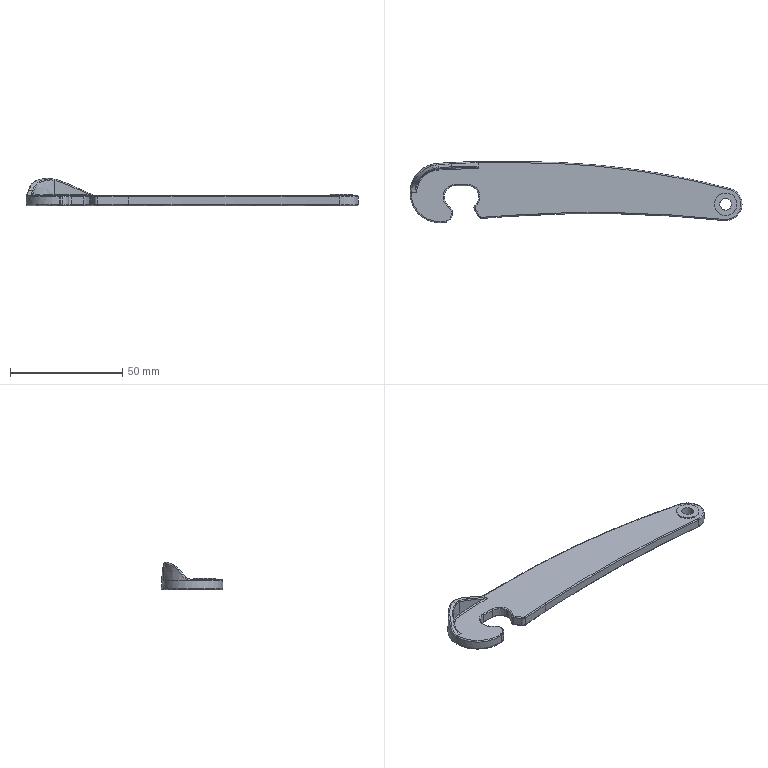Part | SolidWorks | features BaseBody 1 | 1 solid | 131 faces | box 148.137 x 27.348 x 12.258 mm | volume 8368 mm3 | spline 51 | cylinder 51 | plane 25 | cone 4 | commonest cylinder face diameters 1.005 x6 731.909 x5 2.01 x4 10.049 x4 14.076 x3 3.015 x2